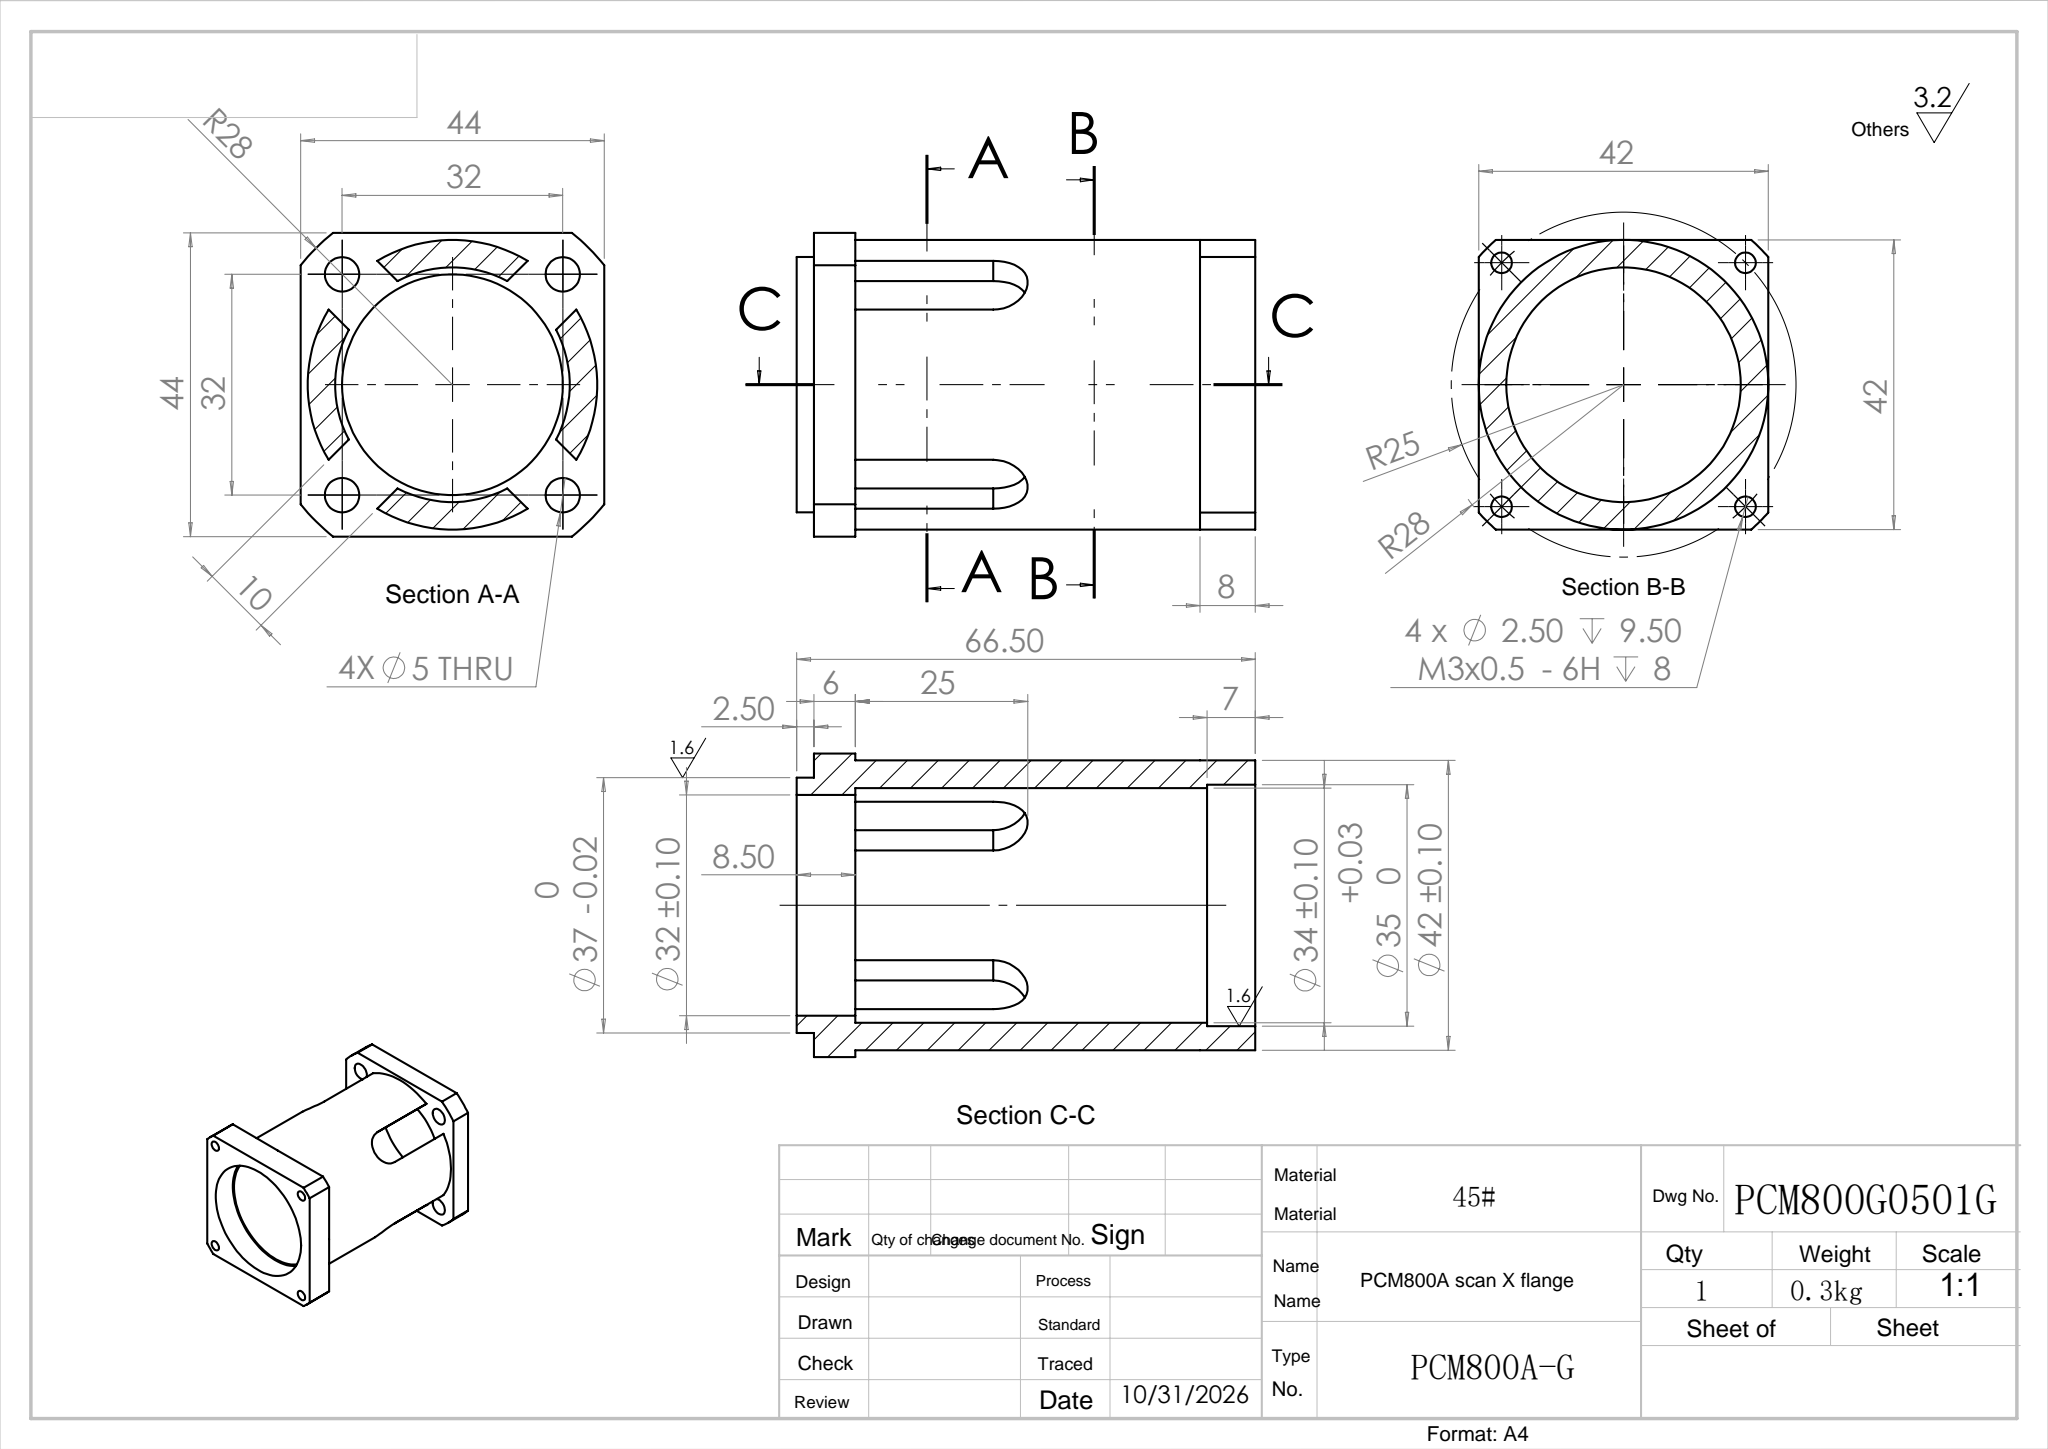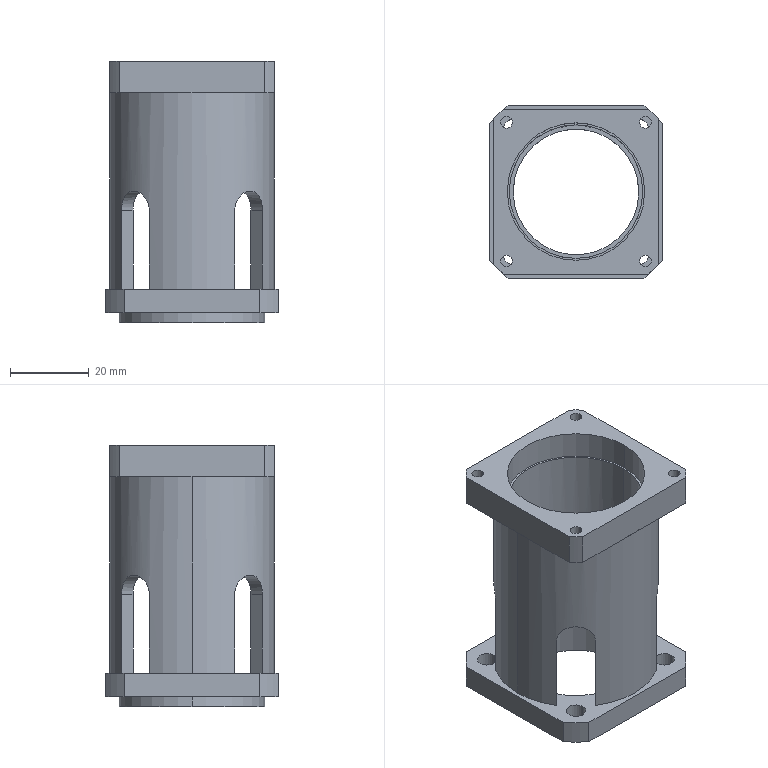Part | SolidWorks | features Cut 7, Boss 3, 3DProfileFeature 1, Extrusion 1, HoleWzd 1 | 1 solid | 63 faces | box 44 x 44 x 66.5 mm | volume 32907 mm3 | cylinder 38 | plane 25 | commonest cylinder face diameters 3 x8 5 x8 56 x8 10 x4 32 x2 34 x2